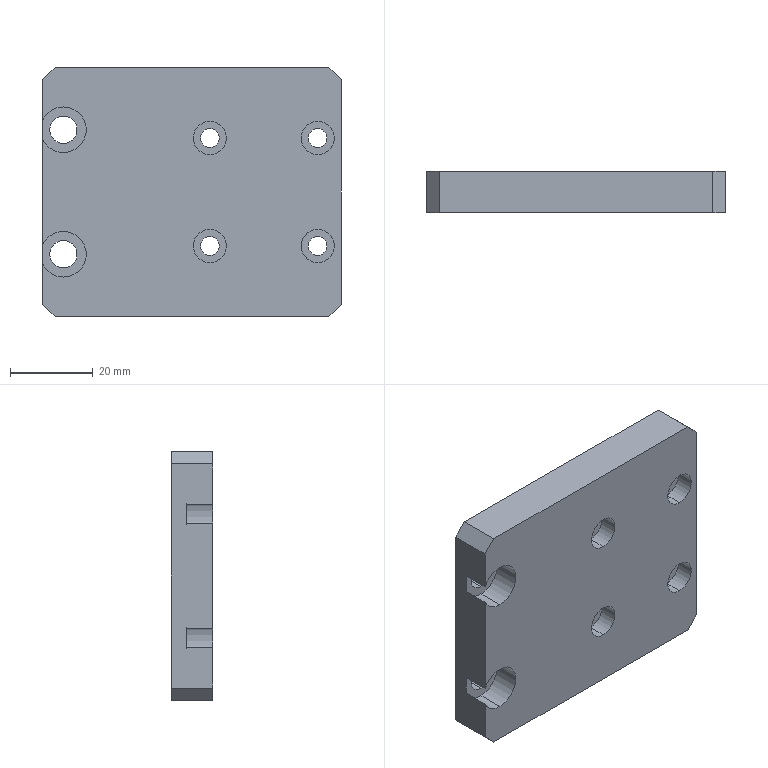Part | SolidWorks | features HoleWzd 4, Chamfer 2, Extrusion 1, ICE 1 | 1 solid | 46 faces | box 72 x 10 x 60 mm | volume 39992 mm3 | cylinder 28 | plane 16 | cone 2 | commonest cylinder face diameters 4.5 x8 8 x8 11 x6 6.6 x4 5 x2
STEP:
#1=CARTESIAN_POINT('',(5.,-44.,18.3));
#2=VERTEX_POINT('',#1);
#3=CARTESIAN_POINT('',(5.,-44.,11.7));
#4=VERTEX_POINT('',#3);
#5=CARTESIAN_POINT('',(5.,-44.,15.));
#6=DIRECTION('',(0.,-1.,0.));
#7=DIRECTION('',(0.,0.,-1.));
#8=AXIS2_PLACEMENT_3D('',#5,#6,#7);
#9=CIRCLE('',#8,3.3);
#10=EDGE_CURVE('',#2,#4,#9,.T.);
#11=ORIENTED_EDGE('',*,*,#10,.F.);
#12=CARTESIAN_POINT('',(5.,-47.6,18.3));
#13=VERTEX_POINT('',#12);
#14=CARTESIAN_POINT('',(5.,-54.,18.3));
#15=DIRECTION('',(0.,-1.,0.));
#16=VECTOR('',#15,1000.);
#17=LINE('',#14,#16);
#18=EDGE_CURVE('',#2,#13,#17,.T.);
#19=ORIENTED_EDGE('',*,*,#18,.T.);
#20=CARTESIAN_POINT('',(5.,-47.6,11.7));
#21=VERTEX_POINT('',#20);
#22=CARTESIAN_POINT('',(5.,-47.6,15.));
#23=DIRECTION('',(0.,-1.,0.));
#24=DIRECTION('',(0.,0.,-1.));
#25=AXIS2_PLACEMENT_3D('',#22,#23,#24);
#26=CIRCLE('',#25,3.3);
#27=EDGE_CURVE('',#13,#21,#26,.T.);
#28=ORIENTED_EDGE('',*,*,#27,.T.);
#29=CARTESIAN_POINT('',(5.,-54.,11.7));
#30=DIRECTION('',(0.,-1.,0.));
#31=VECTOR('',#30,1000.);
#32=LINE('',#29,#31);
#33=EDGE_CURVE('',#4,#21,#32,.T.);
#34=ORIENTED_EDGE('',*,*,#33,.F.);
#35=EDGE_LOOP('',(#11,#19,#28,#34));
#36=FACE_OUTER_BOUND('',#35,.T.);
#37=CARTESIAN_POINT('',(5.,-54.,15.));
#38=DIRECTION('',(0.,-1.,0.));
#39=DIRECTION('',(0.,0.,-1.));
#40=AXIS2_PLACEMENT_3D('',#37,#38,#39);
#41=CYLINDRICAL_SURFACE('',#40,3.3);
#42=ADVANCED_FACE('',(#36),#41,.F.);
#43=CARTESIAN_POINT('',(5.,-47.6,20.5));
#44=VERTEX_POINT('',#43);
#45=CARTESIAN_POINT('',(0.,-47.6,17.291));
#46=VERTEX_POINT('',#45);
#47=CARTESIAN_POINT('',(5.,-47.6,15.));
#48=DIRECTION('',(0.,-1.,0.));
#49=DIRECTION('',(0.,0.,-1.));
#50=AXIS2_PLACEMENT_3D('',#47,#48,#49);
#51=CIRCLE('',#50,5.5);
#52=EDGE_CURVE('',#44,#46,#51,.T.);
#53=ORIENTED_EDGE('',*,*,#52,.F.);
#54=CARTESIAN_POINT('',(5.,-54.,20.5));
#55=VERTEX_POINT('',#54);
#56=CARTESIAN_POINT('',(5.,-54.,20.5));
#57=DIRECTION('',(0.,-1.,0.));
#58=VECTOR('',#57,1000.);
#59=LINE('',#56,#58);
#60=EDGE_CURVE('',#44,#55,#59,.T.);
#61=ORIENTED_EDGE('',*,*,#60,.T.);
#62=CARTESIAN_POINT('',(0.,-54.,17.291));
#63=VERTEX_POINT('',#62);
#64=CARTESIAN_POINT('',(5.,-54.,15.));
#65=DIRECTION('',(0.,1.,0.));
#66=DIRECTION('',(0.,0.,1.));
#67=AXIS2_PLACEMENT_3D('',#64,#65,#66);
#68=CIRCLE('',#67,5.5);
#69=EDGE_CURVE('',#63,#55,#68,.T.);
#70=ORIENTED_EDGE('',*,*,#69,.F.);
#71=CARTESIAN_POINT('',(0.,-54.,17.291));
#72=DIRECTION('',(0.,-1.,0.));
#73=VECTOR('',#72,1000.);
#74=LINE('',#71,#73);
#75=EDGE_CURVE('',#46,#63,#74,.T.);
#76=ORIENTED_EDGE('',*,*,#75,.F.);
#77=EDGE_LOOP('',(#53,#61,#70,#76));
#78=FACE_OUTER_BOUND('',#77,.T.);
#79=CARTESIAN_POINT('',(5.,-54.,15.));
#80=DIRECTION('',(0.,-1.,0.));
#81=DIRECTION('',(0.,0.,-1.));
#82=AXIS2_PLACEMENT_3D('',#79,#80,#81);
#83=CYLINDRICAL_SURFACE('',#82,5.5);
#84=ADVANCED_FACE('',(#78),#83,.F.);
#85=ORIENTED_EDGE('',*,*,#60,.F.);
#86=CARTESIAN_POINT('',(5.,-47.6,9.5));
#87=VERTEX_POINT('',#86);
#88=CARTESIAN_POINT('',(5.,-47.6,15.));
#89=DIRECTION('',(0.,-1.,0.));
#90=DIRECTION('',(0.,0.,-1.));
#91=AXIS2_PLACEMENT_3D('',#88,#89,#90);
#92=CIRCLE('',#91,5.5);
#93=EDGE_CURVE('',#87,#44,#92,.T.);
#94=ORIENTED_EDGE('',*,*,#93,.F.);
#95=CARTESIAN_POINT('',(5.,-54.,9.5));
#96=VERTEX_POINT('',#95);
#97=CARTESIAN_POINT('',(5.,-54.,9.5));
#98=DIRECTION('',(0.,-1.,0.));
#99=VECTOR('',#98,1000.);
#100=LINE('',#97,#99);
#101=EDGE_CURVE('',#87,#96,#100,.T.);
#102=ORIENTED_EDGE('',*,*,#101,.T.);
#103=CARTESIAN_POINT('',(5.,-54.,15.));
#104=DIRECTION('',(0.,1.,0.));
#105=DIRECTION('',(0.,0.,1.));
#106=AXIS2_PLACEMENT_3D('',#103,#104,#105);
#107=CIRCLE('',#106,5.5);
#108=EDGE_CURVE('',#55,#96,#107,.T.);
#109=ORIENTED_EDGE('',*,*,#108,.F.);
#110=EDGE_LOOP('',(#85,#94,#102,#109));
#111=FACE_OUTER_BOUND('',#110,.T.);
#112=CARTESIAN_POINT('',(5.,-54.,15.));
#113=DIRECTION('',(0.,-1.,0.));
#114=DIRECTION('',(0.,0.,-1.));
#115=AXIS2_PLACEMENT_3D('',#112,#113,#114);
#116=CYLINDRICAL_SURFACE('',#115,5.5);
#117=ADVANCED_FACE('',(#111),#116,.F.);
#118=CARTESIAN_POINT('',(5.,-47.6,50.5));
#119=VERTEX_POINT('',#118);
#120=CARTESIAN_POINT('',(0.,-47.6,47.291));
#121=VERTEX_POINT('',#120);
#122=CARTESIAN_POINT('',(5.,-47.6,45.));
#123=DIRECTION('',(0.,-1.,0.));
#124=DIRECTION('',(0.,0.,-1.));
#125=AXIS2_PLACEMENT_3D('',#122,#123,#124);
#126=CIRCLE('',#125,5.5);
#127=EDGE_CURVE('',#119,#121,#126,.T.);
#128=ORIENTED_EDGE('',*,*,#127,.F.);
#129=CARTESIAN_POINT('',(5.,-54.,50.5));
#130=VERTEX_POINT('',#129);
#131=CARTESIAN_POINT('',(5.,-54.,50.5));
#132=DIRECTION('',(0.,-1.,0.));
#133=VECTOR('',#132,1000.);
#134=LINE('',#131,#133);
#135=EDGE_CURVE('',#119,#130,#134,.T.);
#136=ORIENTED_EDGE('',*,*,#135,.T.);
#137=CARTESIAN_POINT('',(0.,-54.,47.291));
#138=VERTEX_POINT('',#137);
#139=CARTESIAN_POINT('',(5.,-54.,45.));
#140=DIRECTION('',(0.,-1.,0.));
#141=DIRECTION('',(0.,0.,-1.));
#142=AXIS2_PLACEMENT_3D('',#139,#140,#141);
#143=CIRCLE('',#142,5.5);
#144=EDGE_CURVE('',#130,#138,#143,.T.);
#145=ORIENTED_EDGE('',*,*,#144,.T.);
#146=CARTESIAN_POINT('',(0.,-54.,47.291));
#147=DIRECTION('',(0.,-1.,0.));
#148=VECTOR('',#147,1000.);
#149=LINE('',#146,#148);
#150=EDGE_CURVE('',#121,#138,#149,.T.);
#151=ORIENTED_EDGE('',*,*,#150,.F.);
#152=EDGE_LOOP('',(#128,#136,#145,#151));
#153=FACE_OUTER_BOUND('',#152,.T.);
#154=CARTESIAN_POINT('',(5.,-54.,45.));
#155=DIRECTION('',(0.,-1.,0.));
#156=DIRECTION('',(0.,0.,-1.));
#157=AXIS2_PLACEMENT_3D('',#154,#155,#156);
#158=CYLINDRICAL_SURFACE('',#157,5.5);
#159=ADVANCED_FACE('',(#153),#158,.F.);
#160=ORIENTED_EDGE('',*,*,#135,.F.);
#161=CARTESIAN_POINT('',(5.,-47.6,39.5));
#162=VERTEX_POINT('',#161);
#163=CARTESIAN_POINT('',(5.,-47.6,45.));
#164=DIRECTION('',(0.,-1.,0.));
#165=DIRECTION('',(0.,0.,-1.));
#166=AXIS2_PLACEMENT_3D('',#163,#164,#165);
#167=CIRCLE('',#166,5.5);
#168=EDGE_CURVE('',#162,#119,#167,.T.);
#169=ORIENTED_EDGE('',*,*,#168,.F.);
#170=CARTESIAN_POINT('',(5.,-54.,39.5));
#171=VERTEX_POINT('',#170);
#172=CARTESIAN_POINT('',(5.,-54.,39.5));
#173=DIRECTION('',(0.,-1.,0.));
#174=VECTOR('',#173,1000.);
#175=LINE('',#172,#174);
#176=EDGE_CURVE('',#162,#171,#175,.T.);
#177=ORIENTED_EDGE('',*,*,#176,.T.);
#178=CARTESIAN_POINT('',(5.,-54.,45.));
#179=DIRECTION('',(0.,-1.,0.));
#180=DIRECTION('',(0.,0.,-1.));
#181=AXIS2_PLACEMENT_3D('',#178,#179,#180);
#182=CIRCLE('',#181,5.5);
#183=EDGE_CURVE('',#171,#130,#182,.T.);
#184=ORIENTED_EDGE('',*,*,#183,.T.);
#185=EDGE_LOOP('',(#160,#169,#177,#184));
#186=FACE_OUTER_BOUND('',#185,.T.);
#187=CARTESIAN_POINT('',(5.,-54.,45.));
#188=DIRECTION('',(0.,-1.,0.));
#189=DIRECTION('',(0.,0.,-1.));
#190=AXIS2_PLACEMENT_3D('',#187,#188,#189);
#191=CYLINDRICAL_SURFACE('',#190,5.5);
#192=ADVANCED_FACE('',(#186),#191,.F.);
#193=CARTESIAN_POINT('',(5.,-44.,48.3));
#194=VERTEX_POINT('',#193);
#195=CARTESIAN_POINT('',(5.,-44.,41.7));
#196=VERTEX_POINT('',#195);
#197=CARTESIAN_POINT('',(5.,-44.,45.));
#198=DIRECTION('',(0.,-1.,0.));
#199=DIRECTION('',(0.,0.,-1.));
#200=AXIS2_PLACEMENT_3D('',#197,#198,#199);
#201=CIRCLE('',#200,3.3);
#202=EDGE_CURVE('',#194,#196,#201,.T.);
#203=ORIENTED_EDGE('',*,*,#202,.F.);
#204=CARTESIAN_POINT('',(5.,-47.6,48.3));
#205=VERTEX_POINT('',#204);
#206=CARTESIAN_POINT('',(5.,-54.,48.3));
#207=DIRECTION('',(0.,-1.,0.));
#208=VECTOR('',#207,1000.);
#209=LINE('',#206,#208);
#210=EDGE_CURVE('',#194,#205,#209,.T.);
#211=ORIENTED_EDGE('',*,*,#210,.T.);
#212=CARTESIAN_POINT('',(5.,-47.6,41.7));
#213=VERTEX_POINT('',#212);
#214=CARTESIAN_POINT('',(5.,-47.6,45.));
#215=DIRECTION('',(0.,-1.,0.));
#216=DIRECTION('',(0.,0.,-1.));
#217=AXIS2_PLACEMENT_3D('',#214,#215,#216);
#218=CIRCLE('',#217,3.3);
#219=EDGE_CURVE('',#205,#213,#218,.T.);
#220=ORIENTED_EDGE('',*,*,#219,.T.);
#221=CARTESIAN_POINT('',(5.,-54.,41.7));
#222=DIRECTION('',(0.,-1.,0.));
#223=VECTOR('',#222,1000.);
#224=LINE('',#221,#223);
#225=EDGE_CURVE('',#196,#213,#224,.T.);
#226=ORIENTED_EDGE('',*,*,#225,.F.);
#227=EDGE_LOOP('',(#203,#211,#220,#226));
#228=FACE_OUTER_BOUND('',#227,.T.);
#229=CARTESIAN_POINT('',(5.,-54.,45.));
#230=DIRECTION('',(0.,-1.,0.));
#231=DIRECTION('',(0.,0.,-1.));
#232=AXIS2_PLACEMENT_3D('',#229,#230,#231);
#233=CYLINDRICAL_SURFACE('',#232,3.3);
#234=ADVANCED_FACE('',(#228),#233,.F.);
#235=CARTESIAN_POINT('',(40.3,-49.6,21.));
#236=VERTEX_POINT('',#235);
#237=CARTESIAN_POINT('',(40.3,-49.6,13.));
#238=VERTEX_POINT('',#237);
#239=CARTESIAN_POINT('',(40.3,-49.6,17.));
#240=DIRECTION('',(0.,-1.,0.));
#241=DIRECTION('',(0.,0.,-1.));
#242=AXIS2_PLACEMENT_3D('',#239,#240,#241);
#243=CIRCLE('',#242,4.);
#244=EDGE_CURVE('',#236,#238,#243,.T.);
#245=ORIENTED_EDGE('',*,*,#244,.F.);
#246=CARTESIAN_POINT('',(40.3,-54.,21.));
#247=VERTEX_POINT('',#246);
#248=CARTESIAN_POINT('',(40.3,-54.,21.));
#249=DIRECTION('',(0.,-1.,0.));
#250=VECTOR('',#249,1000.);
#251=LINE('',#248,#250);
#252=EDGE_CURVE('',#236,#247,#251,.T.);
#253=ORIENTED_EDGE('',*,*,#252,.T.);
#254=CARTESIAN_POINT('',(40.3,-54.,13.));
#255=VERTEX_POINT('',#254);
#256=CARTESIAN_POINT('',(40.3,-54.,17.));
#257=DIRECTION('',(0.,-1.,0.));
#258=DIRECTION('',(0.,0.,-1.));
#259=AXIS2_PLACEMENT_3D('',#256,#257,#258);
#260=CIRCLE('',#259,4.);
#261=EDGE_CURVE('',#247,#255,#260,.T.);
#262=ORIENTED_EDGE('',*,*,#261,.T.);
#263=CARTESIAN_POINT('',(40.3,-54.,13.));
#264=DIRECTION('',(0.,-1.,0.));
#265=VECTOR('',#264,1000.);
#266=LINE('',#263,#265);
#267=EDGE_CURVE('',#238,#255,#266,.T.);
#268=ORIENTED_EDGE('',*,*,#267,.F.);
#269=EDGE_LOOP('',(#245,#253,#262,#268));
#270=FACE_OUTER_BOUND('',#269,.T.);
#271=CARTESIAN_POINT('',(40.3,-54.,17.));
#272=DIRECTION('',(0.,-1.,0.));
#273=DIRECTION('',(0.,0.,-1.));
#274=AXIS2_PLACEMENT_3D('',#271,#272,#273);
#275=CYLINDRICAL_SURFACE('',#274,4.);
#276=ADVANCED_FACE('',(#270),#275,.F.);
#277=CARTESIAN_POINT('',(40.3,-44.,19.25));
#278=VERTEX_POINT('',#277);
#279=CARTESIAN_POINT('',(40.3,-44.,14.75));
#280=VERTEX_POINT('',#279);
#281=CARTESIAN_POINT('',(40.3,-44.,17.));
#282=DIRECTION('',(0.,-1.,0.));
#283=DIRECTION('',(0.,0.,-1.));
#284=AXIS2_PLACEMENT_3D('',#281,#282,#283);
#285=CIRCLE('',#284,2.25);
#286=EDGE_CURVE('',#278,#280,#285,.T.);
#287=ORIENTED_EDGE('',*,*,#286,.F.);
#288=CARTESIAN_POINT('',(40.3,-49.6,19.25));
#289=VERTEX_POINT('',#288);
#290=CARTESIAN_POINT('',(40.3,-54.,19.25));
#291=DIRECTION('',(0.,-1.,0.));
#292=VECTOR('',#291,1000.);
#293=LINE('',#290,#292);
#294=EDGE_CURVE('',#278,#289,#293,.T.);
#295=ORIENTED_EDGE('',*,*,#294,.T.);
#296=CARTESIAN_POINT('',(40.3,-49.6,14.75));
#297=VERTEX_POINT('',#296);
#298=CARTESIAN_POINT('',(40.3,-49.6,17.));
#299=DIRECTION('',(0.,-1.,0.));
#300=DIRECTION('',(0.,0.,-1.));
#301=AXIS2_PLACEMENT_3D('',#298,#299,#300);
#302=CIRCLE('',#301,2.25);
#303=EDGE_CURVE('',#289,#297,#302,.T.);
#304=ORIENTED_EDGE('',*,*,#303,.T.);
#305=CARTESIAN_POINT('',(40.3,-54.,14.75));
#306=DIRECTION('',(0.,-1.,0.));
#307=VECTOR('',#306,1000.);
#308=LINE('',#305,#307);
#309=EDGE_CURVE('',#280,#297,#308,.T.);
#310=ORIENTED_EDGE('',*,*,#309,.F.);
#311=EDGE_LOOP('',(#287,#295,#304,#310));
#312=FACE_OUTER_BOUND('',#311,.T.);
#313=CARTESIAN_POINT('',(40.3,-54.,17.));
#314=DIRECTION('',(0.,-1.,0.));
#315=DIRECTION('',(0.,0.,-1.));
#316=AXIS2_PLACEMENT_3D('',#313,#314,#315);
#317=CYLINDRICAL_SURFACE('',#316,2.25);
#318=ADVANCED_FACE('',(#312),#317,.F.);
#319=CARTESIAN_POINT('',(66.3,-49.6,21.));
#320=VERTEX_POINT('',#319);
#321=CARTESIAN_POINT('',(62.301,-49.6,17.074));
#322=VERTEX_POINT('',#321);
#323=CARTESIAN_POINT('',(66.3,-49.6,17.));
#324=DIRECTION('',(0.,-1.,0.));
#325=DIRECTION('',(0.,0.,-1.));
#326=AXIS2_PLACEMENT_3D('',#323,#324,#325);
#327=CIRCLE('',#326,4.);
#328=EDGE_CURVE('',#320,#322,#327,.T.);
#329=ORIENTED_EDGE('',*,*,#328,.F.);
#330=CARTESIAN_POINT('',(66.3,-54.,21.));
#331=VERTEX_POINT('',#330);
#332=CARTESIAN_POINT('',(66.3,-54.,21.));
#333=DIRECTION('',(0.,-1.,0.));
#334=VECTOR('',#333,1000.);
#335=LINE('',#332,#334);
#336=EDGE_CURVE('',#320,#331,#335,.T.);
#337=ORIENTED_EDGE('',*,*,#336,.T.);
#338=CARTESIAN_POINT('',(66.3,-54.,13.));
#339=VERTEX_POINT('',#338);
#340=CARTESIAN_POINT('',(66.3,-54.,17.));
#341=DIRECTION('',(0.,-1.,0.));
#342=DIRECTION('',(0.,0.,-1.));
#343=AXIS2_PLACEMENT_3D('',#340,#341,#342);
#344=CIRCLE('',#343,4.);
#345=EDGE_CURVE('',#331,#339,#344,.T.);
#346=ORIENTED_EDGE('',*,*,#345,.T.);
#347=CARTESIAN_POINT('',(66.3,-49.6,13.));
#348=VERTEX_POINT('',#347);
#349=CARTESIAN_POINT('',(66.3,-54.,13.));
#350=DIRECTION('',(0.,-1.,0.));
#351=VECTOR('',#350,1000.);
#352=LINE('',#349,#351);
#353=EDGE_CURVE('',#348,#339,#352,.T.);
#354=ORIENTED_EDGE('',*,*,#353,.F.);
#355=CARTESIAN_POINT('',(62.427,-49.6,16.));
#356=VERTEX_POINT('',#355);
#357=CARTESIAN_POINT('',(66.3,-49.6,17.));
#358=DIRECTION('',(0.,-1.,0.));
#359=DIRECTION('',(0.,0.,-1.));
#360=AXIS2_PLACEMENT_3D('',#357,#358,#359);
#361=CIRCLE('',#360,4.);
#362=EDGE_CURVE('',#356,#348,#361,.T.);
#363=ORIENTED_EDGE('',*,*,#362,.F.);
#364=CARTESIAN_POINT('',(62.3,-49.98,17.));
#365=VERTEX_POINT('',#364);
#366=CARTESIAN_POINT('',(62.3,-49.98,17.));
#367=CARTESIAN_POINT('',(62.3,-49.98,16.907));
#368=CARTESIAN_POINT('',(62.303,-49.972,16.815));
#369=CARTESIAN_POINT('',(62.316,-49.942,16.635));
#370=CARTESIAN_POINT('',(62.325,-49.919,16.544));
#371=CARTESIAN_POINT('',(62.349,-49.858,16.373));
#372=CARTESIAN_POINT('',(62.363,-49.819,16.291));
#373=CARTESIAN_POINT('',(62.394,-49.723,16.136));
#374=CARTESIAN_POINT('',(62.411,-49.666,16.064));
#375=CARTESIAN_POINT('',(62.427,-49.6,16.));
#376=B_SPLINE_CURVE_WITH_KNOTS('',3,(#366,#367,#368,#369,#370,#371,#372,#373,#374,#375),.UNSPECIFIED.,.F.,.F.,(4,2,2,2,4),(0.,0.0002756,0.0005511,0.0008267,0.001102),.UNSPECIFIED.);
#377=EDGE_CURVE('',#365,#356,#376,.T.);
#378=ORIENTED_EDGE('',*,*,#377,.F.);
#379=CARTESIAN_POINT('',(62.301,-49.6,17.074));
#380=CARTESIAN_POINT('',(62.3,-49.728,17.054));
#381=CARTESIAN_POINT('',(62.3,-49.854,17.03));
#382=CARTESIAN_POINT('',(62.3,-49.98,17.));
#383=B_SPLINE_CURVE_WITH_KNOTS('',3,(#379,#380,#381,#382),.UNSPECIFIED.,.F.,.F.,(4,4),(0.0001908,0.0005775),.UNSPECIFIED.);
#384=EDGE_CURVE('',#322,#365,#383,.T.);
#385=ORIENTED_EDGE('',*,*,#384,.F.);
#386=EDGE_LOOP('',(#329,#337,#346,#354,#363,#378,#385));
#387=FACE_OUTER_BOUND('',#386,.T.);
#388=CARTESIAN_POINT('',(66.3,-54.,17.));
#389=DIRECTION('',(0.,-1.,0.));
#390=DIRECTION('',(0.,0.,-1.));
#391=AXIS2_PLACEMENT_3D('',#388,#389,#390);
#392=CYLINDRICAL_SURFACE('',#391,4.);
#393=ADVANCED_FACE('',(#387),#392,.F.);
#394=CARTESIAN_POINT('',(66.3,-44.,19.25));
#395=VERTEX_POINT('',#394);
#396=CARTESIAN_POINT('',(66.3,-44.,14.75));
#397=VERTEX_POINT('',#396);
#398=CARTESIAN_POINT('',(66.3,-44.,17.));
#399=DIRECTION('',(0.,-1.,0.));
#400=DIRECTION('',(0.,0.,-1.));
#401=AXIS2_PLACEMENT_3D('',#398,#399,#400);
#402=CIRCLE('',#401,2.25);
#403=EDGE_CURVE('',#395,#397,#402,.T.);
#404=ORIENTED_EDGE('',*,*,#403,.F.);
#405=CARTESIAN_POINT('',(66.3,-49.6,19.25));
#406=VERTEX_POINT('',#405);
#407=CARTESIAN_POINT('',(66.3,-54.,19.25));
#408=DIRECTION('',(0.,-1.,0.));
#409=VECTOR('',#408,1000.);
#410=LINE('',#407,#409);
#411=EDGE_CURVE('',#395,#406,#410,.T.);
#412=ORIENTED_EDGE('',*,*,#411,.T.);
#413=CARTESIAN_POINT('',(66.3,-49.6,14.75));
#414=VERTEX_POINT('',#413);
#415=CARTESIAN_POINT('',(66.3,-49.6,17.));
#416=DIRECTION('',(0.,-1.,0.));
#417=DIRECTION('',(0.,0.,-1.));
#418=AXIS2_PLACEMENT_3D('',#415,#416,#417);
#419=CIRCLE('',#418,2.25);
#420=EDGE_CURVE('',#406,#414,#419,.T.);
#421=ORIENTED_EDGE('',*,*,#420,.T.);
#422=CARTESIAN_POINT('',(66.3,-54.,14.75));
#423=DIRECTION('',(0.,-1.,0.));
#424=VECTOR('',#423,1000.);
#425=LINE('',#422,#424);
#426=EDGE_CURVE('',#397,#414,#425,.T.);
#427=ORIENTED_EDGE('',*,*,#426,.F.);
#428=EDGE_LOOP('',(#404,#412,#421,#427));
#429=FACE_OUTER_BOUND('',#428,.T.);
#430=CARTESIAN_POINT('',(66.3,-54.,17.));
#431=DIRECTION('',(0.,-1.,0.));
#432=DIRECTION('',(0.,0.,-1.));
#433=AXIS2_PLACEMENT_3D('',#430,#431,#432);
#434=CYLINDRICAL_SURFACE('',#433,2.25);
#435=ADVANCED_FACE('',(#429),#434,.F.);
#436=CARTESIAN_POINT('',(66.3,-49.6,47.));
#437=VERTEX_POINT('',#436);
#438=CARTESIAN_POINT('',(66.3,-49.6,39.));
#439=VERTEX_POINT('',#438);
#440=CARTESIAN_POINT('',(66.3,-49.6,43.));
#441=DIRECTION('',(0.,-1.,0.));
#442=DIRECTION('',(0.,0.,-1.));
#443=AXIS2_PLACEMENT_3D('',#440,#441,#442);
#444=CIRCLE('',#443,4.);
#445=EDGE_CURVE('',#437,#439,#444,.T.);
#446=ORIENTED_EDGE('',*,*,#445,.F.);
#447=CARTESIAN_POINT('',(66.3,-54.,47.));
#448=VERTEX_POINT('',#447);
#449=CARTESIAN_POINT('',(66.3,-54.,47.));
#450=DIRECTION('',(0.,-1.,0.));
#451=VECTOR('',#450,1000.);
#452=LINE('',#449,#451);
#453=EDGE_CURVE('',#437,#448,#452,.T.);
#454=ORIENTED_EDGE('',*,*,#453,.T.);
#455=CARTESIAN_POINT('',(66.3,-54.,39.));
#456=VERTEX_POINT('',#455);
#457=CARTESIAN_POINT('',(66.3,-54.,43.));
#458=DIRECTION('',(0.,-1.,0.));
#459=DIRECTION('',(0.,0.,-1.));
#460=AXIS2_PLACEMENT_3D('',#457,#458,#459);
#461=CIRCLE('',#460,4.);
#462=EDGE_CURVE('',#448,#456,#461,.T.);
#463=ORIENTED_EDGE('',*,*,#462,.T.);
#464=CARTESIAN_POINT('',(66.3,-54.,39.));
#465=DIRECTION('',(0.,-1.,0.));
#466=VECTOR('',#465,1000.);
#467=LINE('',#464,#466);
#468=EDGE_CURVE('',#439,#456,#467,.T.);
#469=ORIENTED_EDGE('',*,*,#468,.F.);
#470=EDGE_LOOP('',(#446,#454,#463,#469));
#471=FACE_OUTER_BOUND('',#470,.T.);
#472=CARTESIAN_POINT('',(66.3,-54.,43.));
#473=DIRECTION('',(0.,-1.,0.));
#474=DIRECTION('',(0.,0.,-1.));
#475=AXIS2_PLACEMENT_3D('',#472,#473,#474);
#476=CYLINDRICAL_SURFACE('',#475,4.);
#477=ADVANCED_FACE('',(#471),#476,.F.);
#478=CARTESIAN_POINT('',(66.3,-44.,45.25));
#479=VERTEX_POINT('',#478);
#480=CARTESIAN_POINT('',(66.3,-44.,40.75));
#481=VERTEX_POINT('',#480);
#482=CARTESIAN_POINT('',(66.3,-44.,43.));
#483=DIRECTION('',(0.,-1.,0.));
#484=DIRECTION('',(0.,0.,-1.));
#485=AXIS2_PLACEMENT_3D('',#482,#483,#484);
#486=CIRCLE('',#485,2.25);
#487=EDGE_CURVE('',#479,#481,#486,.T.);
#488=ORIENTED_EDGE('',*,*,#487,.F.);
#489=CARTESIAN_POINT('',(66.3,-49.6,45.25));
#490=VERTEX_POINT('',#489);
#491=CARTESIAN_POINT('',(66.3,-54.,45.25));
#492=DIRECTION('',(0.,-1.,0.));
#493=VECTOR('',#492,1000.);
#494=LINE('',#491,#493);
#495=EDGE_CURVE('',#479,#490,#494,.T.);
#496=ORIENTED_EDGE('',*,*,#495,.T.);
#497=CARTESIAN_POINT('',(66.3,-49.6,40.75));
#498=VERTEX_POINT('',#497);
#499=CARTESIAN_POINT('',(66.3,-49.6,43.));
#500=DIRECTION('',(0.,-1.,0.));
#501=DIRECTION('',(0.,0.,-1.));
#502=AXIS2_PLACEMENT_3D('',#499,#500,#501);
#503=CIRCLE('',#502,2.25);
#504=EDGE_CURVE('',#490,#498,#503,.T.);
#505=ORIENTED_EDGE('',*,*,#504,.T.);
#506=CARTESIAN_POINT('',(66.3,-54.,40.75));
#507=DIRECTION('',(0.,-1.,0.));
#508=VECTOR('',#507,1000.);
#509=LINE('',#506,#508);
#510=EDGE_CURVE('',#481,#498,#509,.T.);
#511=ORIENTED_EDGE('',*,*,#510,.F.);
#512=EDGE_LOOP('',(#488,#496,#505,#511));
#513=FACE_OUTER_BOUND('',#512,.T.);
#514=CARTESIAN_POINT('',(66.3,-54.,43.));
#515=DIRECTION('',(0.,-1.,0.));
#516=DIRECTION('',(0.,0.,-1.));
#517=AXIS2_PLACEMENT_3D('',#514,#515,#516);
#518=CYLINDRICAL_SURFACE('',#517,2.25);
#519=ADVANCED_FACE('',(#513),#518,.F.);
#520=CARTESIAN_POINT('',(40.3,-49.6,47.));
#521=VERTEX_POINT('',#520);
#522=CARTESIAN_POINT('',(40.3,-49.6,39.));
#523=VERTEX_POINT('',#522);
#524=CARTESIAN_POINT('',(40.3,-49.6,43.));
#525=DIRECTION('',(0.,-1.,0.));
#526=DIRECTION('',(0.,0.,-1.));
#527=AXIS2_PLACEMENT_3D('',#524,#525,#526);
#528=CIRCLE('',#527,4.);
#529=EDGE_CURVE('',#521,#523,#528,.T.);
#530=ORIENTED_EDGE('',*,*,#529,.F.);
#531=CARTESIAN_POINT('',(40.3,-54.,47.));
#532=VERTEX_POINT('',#531);
#533=CARTESIAN_POINT('',(40.3,-54.,47.));
#534=DIRECTION('',(0.,-1.,0.));
#535=VECTOR('',#534,1000.);
#536=LINE('',#533,#535);
#537=EDGE_CURVE('',#521,#532,#536,.T.);
#538=ORIENTED_EDGE('',*,*,#537,.T.);
#539=CARTESIAN_POINT('',(40.3,-54.,39.));
#540=VERTEX_POINT('',#539);
#541=CARTESIAN_POINT('',(40.3,-54.,43.));
#542=DIRECTION('',(0.,-1.,0.));
#543=DIRECTION('',(0.,0.,-1.));
#544=AXIS2_PLACEMENT_3D('',#541,#542,#543);
#545=CIRCLE('',#544,4.);
#546=EDGE_CURVE('',#532,#540,#545,.T.);
#547=ORIENTED_EDGE('',*,*,#546,.T.);
#548=CARTESIAN_POINT('',(40.3,-54.,39.));
#549=DIRECTION('',(0.,-1.,0.));
#550=VECTOR('',#549,1000.);
#551=LINE('',#548,#550);
#552=EDGE_CURVE('',#523,#540,#551,.T.);
#553=ORIENTED_EDGE('',*,*,#552,.F.);
#554=EDGE_LOOP('',(#530,#538,#547,#553));
#555=FACE_OUTER_BOUND('',#554,.T.);
#556=CARTESIAN_POINT('',(40.3,-54.,43.));
#557=DIRECTION('',(0.,-1.,0.));
#558=DIRECTION('',(0.,0.,-1.));
#559=AXIS2_PLACEMENT_3D('',#556,#557,#558);
#560=CYLINDRICAL_SURFACE('',#559,4.);
#561=ADVANCED_FACE('',(#555),#560,.F.);
#562=CARTESIAN_POINT('',(40.3,-44.,45.25));
#563=VERTEX_POINT('',#562);
#564=CARTESIAN_POINT('',(40.3,-44.,40.75));
#565=VERTEX_POINT('',#564);
#566=CARTESIAN_POINT('',(40.3,-44.,43.));
#567=DIRECTION('',(0.,-1.,0.));
#568=DIRECTION('',(0.,0.,-1.));
#569=AXIS2_PLACEMENT_3D('',#566,#567,#568);
#570=CIRCLE('',#569,2.25);
#571=EDGE_CURVE('',#563,#565,#570,.T.);
#572=ORIENTED_EDGE('',*,*,#571,.F.);
#573=CARTESIAN_POINT('',(40.3,-49.6,45.25));
#574=VERTEX_POINT('',#573);
#575=CARTESIAN_POINT('',(40.3,-54.,45.25));
#576=DIRECTION('',(0.,-1.,0.));
#577=VECTOR('',#576,1000.);
#578=LINE('',#575,#577);
#579=EDGE_CURVE('',#563,#574,#578,.T.);
#580=ORIENTED_EDGE('',*,*,#579,.T.);
#581=CARTESIAN_POINT('',(40.3,-49.6,40.75));
#582=VERTEX_POINT('',#581);
#583=CARTESIAN_POINT('',(40.3,-49.6,43.));
#584=DIRECTION('',(0.,-1.,0.));
#585=DIRECTION('',(0.,0.,-1.));
#586=AXIS2_PLACEMENT_3D('',#583,#584,#585);
#587=CIRCLE('',#586,2.25);
#588=EDGE_CURVE('',#574,#582,#587,.T.);
#589=ORIENTED_EDGE('',*,*,#588,.T.);
#590=CARTESIAN_POINT('',(40.3,-54.,40.75));
#591=DIRECTION('',(0.,-1.,0.));
#592=VECTOR('',#591,1000.);
#593=LINE('',#590,#592);
#594=EDGE_CURVE('',#565,#582,#593,.T.);
#595=ORIENTED_EDGE('',*,*,#594,.F.);
#596=EDGE_LOOP('',(#572,#580,#589,#595));
#597=FACE_OUTER_BOUND('',#596,.T.);
#598=CARTESIAN_POINT('',(40.3,-54.,43.));
#599=DIRECTION('',(0.,-1.,0.));
#600=DIRECTION('',(0.,0.,-1.));
#601=AXIS2_PLACEMENT_3D('',#598,#599,#600);
#602=CYLINDRICAL_SURFACE('',#601,2.25);
#603=ADVANCED_FACE('',(#597),#602,.F.);
#604=CARTESIAN_POINT('',(62.5,-49.,17.));
#605=VERTEX_POINT('',#604);
#606=CARTESIAN_POINT('',(62.427,-49.6,17.));
#607=VERTEX_POINT('',#606);
#608=CARTESIAN_POINT('',(60.,-49.,17.));
#609=DIRECTION('',(0.,0.,-1.));
#610=DIRECTION('',(-1.,0.,0.));
#611=AXIS2_PLACEMENT_3D('',#608,#609,#610);
#612=CIRCLE('',#611,2.5);
#613=EDGE_CURVE('',#605,#607,#612,.T.);
#614=ORIENTED_EDGE('',*,*,#613,.F.);
#615=CARTESIAN_POINT('',(62.5,-49.,0.));
#616=VERTEX_POINT('',#615);
#617=CARTESIAN_POINT('',(62.5,-49.,0.));
#618=DIRECTION('',(0.,0.,-1.));
#619=VECTOR('',#618,1000.);
#620=LINE('',#617,#619);
#621=EDGE_CURVE('',#605,#616,#620,.T.);
#622=ORIENTED_EDGE('',*,*,#621,.T.);
#623=CARTESIAN_POINT('',(57.5,-49.,0.));
#624=VERTEX_POINT('',#623);
#625=CARTESIAN_POINT('',(60.,-49.,0.));
#626=DIRECTION('',(0.,0.,-1.));
#627=DIRECTION('',(-1.,0.,0.));
#628=AXIS2_PLACEMENT_3D('',#625,#626,#627);
#629=CIRCLE('',#628,2.5);
#630=EDGE_CURVE('',#616,#624,#629,.T.);
#631=ORIENTED_EDGE('',*,*,#630,.T.);
#632=CARTESIAN_POINT('',(57.5,-49.,17.));
#633=VERTEX_POINT('',#632);
#634=CARTESIAN_POINT('',(57.5,-49.,0.));
#635=DIRECTION('',(0.,0.,-1.));
#636=VECTOR('',#635,1000.);
#637=LINE('',#634,#636);
#638=EDGE_CURVE('',#633,#624,#637,.T.);
#639=ORIENTED_EDGE('',*,*,#638,.F.);
#640=CARTESIAN_POINT('',(60.,-49.,17.));
#641=DIRECTION('',(0.,0.,-1.));
#642=DIRECTION('',(-1.,0.,0.));
#643=AXIS2_PLACEMENT_3D('',#640,#641,#642);
#644=CIRCLE('',#643,2.5);
#645=EDGE_CURVE('',#365,#633,#644,.T.);
#646=ORIENTED_EDGE('',*,*,#645,.F.);
#647=ORIENTED_EDGE('',*,*,#377,.T.);
#648=CARTESIAN_POINT('',(62.427,-49.6,0.));
#649=DIRECTION('',(0.,0.,1.));
#650=VECTOR('',#649,1000.);
#651=LINE('',#648,#650);
#652=EDGE_CURVE('',#356,#607,#651,.T.);
#653=ORIENTED_EDGE('',*,*,#652,.T.);
#654=EDGE_LOOP('',(#614,#622,#631,#639,#646,#647,#653));
#655=FACE_OUTER_BOUND('',#654,.T.);
#656=CARTESIAN_POINT('',(60.,-49.,0.));
#657=DIRECTION('',(0.,0.,-1.));
#658=DIRECTION('',(-1.,0.,0.));
#659=AXIS2_PLACEMENT_3D('',#656,#657,#658);
#660=CYLINDRICAL_SURFACE('',#659,2.5);
#661=ADVANCED_FACE('',(#655),#660,.F.);
#662=CARTESIAN_POINT('',(60.,-49.,18.502));
#663=VERTEX_POINT('',#662);
#664=CARTESIAN_POINT('',(57.5,-49.,17.));
#665=DIRECTION('',(-0.8572,0.,-0.515));
#666=VECTOR('',#665,1000.);
#667=LINE('',#664,#666);
#668=EDGE_CURVE('',#663,#633,#667,.T.);
#669=ORIENTED_EDGE('',*,*,#668,.F.);
#670=CARTESIAN_POINT('',(62.5,-49.,17.));
#671=DIRECTION('',(0.8572,0.,-0.515));
#672=VECTOR('',#671,1000.);
#673=LINE('',#670,#672);
#674=EDGE_CURVE('',#663,#605,#673,.T.);
#675=ORIENTED_EDGE('',*,*,#674,.T.);
#676=ORIENTED_EDGE('',*,*,#613,.T.);
#677=CARTESIAN_POINT('',(62.427,-49.6,17.));
#678=CARTESIAN_POINT('',(62.385,-49.6,17.025));
#679=CARTESIAN_POINT('',(62.343,-49.6,17.049));
#680=CARTESIAN_POINT('',(62.301,-49.6,17.074));
#681=B_SPLINE_CURVE_WITH_KNOTS('',3,(#677,#678,#679,#680),.UNSPECIFIED.,.F.,.F.,(4,4),(0.002652,0.002798),.UNSPECIFIED.);
#682=EDGE_CURVE('',#607,#322,#681,.T.);
#683=ORIENTED_EDGE('',*,*,#682,.T.);
#684=ORIENTED_EDGE('',*,*,#384,.T.);
#685=ORIENTED_EDGE('',*,*,#645,.T.);
#686=EDGE_LOOP('',(#669,#675,#676,#683,#684,#685));
#687=FACE_OUTER_BOUND('',#686,.T.);
#688=CARTESIAN_POINT('',(60.,-49.,17.));
#689=DIRECTION('',(0.,0.,-1.));
#690=DIRECTION('',(-1.,0.,0.));
#691=AXIS2_PLACEMENT_3D('',#688,#689,#690);
#692=CONICAL_SURFACE('',#691,2.5,1.03);
#693=ADVANCED_FACE('',(#687),#692,.F.);
#694=CARTESIAN_POINT('',(40.3,-54.,17.));
#695=DIRECTION('',(0.,-1.,0.));
#696=DIRECTION('',(0.,0.,-1.));
#697=AXIS2_PLACEMENT_3D('',#694,#695,#696);
#698=CIRCLE('',#697,4.);
#699=EDGE_CURVE('',#255,#247,#698,.T.);
#700=ORIENTED_EDGE('',*,*,#699,.F.);
#701=ORIENTED_EDGE('',*,*,#261,.F.);
#702=EDGE_LOOP('',(#700,#701));
#703=FACE_BOUND('',#702,.T.);
#704=CARTESIAN_POINT('',(66.3,-54.,17.));
#705=DIRECTION('',(0.,-1.,0.));
#706=DIRECTION('',(0.,0.,-1.));
#707=AXIS2_PLACEMENT_3D('',#704,#705,#706);
#708=CIRCLE('',#707,4.);
#709=EDGE_CURVE('',#339,#331,#708,.T.);
#710=ORIENTED_EDGE('',*,*,#709,.F.);
#711=ORIENTED_EDGE('',*,*,#345,.F.);
#712=EDGE_LOOP('',(#710,#711));
#713=FACE_BOUND('',#712,.T.);
#714=CARTESIAN_POINT('',(66.3,-54.,43.));
#715=DIRECTION('',(0.,-1.,0.));
#716=DIRECTION('',(0.,0.,-1.));
#717=AXIS2_PLACEMENT_3D('',#714,#715,#716);
#718=CIRCLE('',#717,4.);
#719=EDGE_CURVE('',#456,#448,#718,.T.);
#720=ORIENTED_EDGE('',*,*,#719,.F.);
#721=ORIENTED_EDGE('',*,*,#462,.F.);
#722=EDGE_LOOP('',(#720,#721));
#723=FACE_BOUND('',#722,.T.);
#724=CARTESIAN_POINT('',(0.,-54.,42.709));
#725=VERTEX_POINT('',#724);
#726=CARTESIAN_POINT('',(0.,-54.,60.));
#727=DIRECTION('',(0.,0.,-1.));
#728=VECTOR('',#727,1000.);
#729=LINE('',#726,#728);
#730=EDGE_CURVE('',#725,#63,#729,.T.);
#731=ORIENTED_EDGE('',*,*,#730,.T.);
#732=ORIENTED_EDGE('',*,*,#69,.T.);
#733=ORIENTED_EDGE('',*,*,#108,.T.);
#734=CARTESIAN_POINT('',(0.,-54.,12.709));
#735=VERTEX_POINT('',#734);
#736=CARTESIAN_POINT('',(5.,-54.,15.));
#737=DIRECTION('',(0.,1.,0.));
#738=DIRECTION('',(0.,0.,1.));
#739=AXIS2_PLACEMENT_3D('',#736,#737,#738);
#740=CIRCLE('',#739,5.5);
#741=EDGE_CURVE('',#96,#735,#740,.T.);
#742=ORIENTED_EDGE('',*,*,#741,.T.);
#743=CARTESIAN_POINT('',(0.,-54.,3.));
#744=VERTEX_POINT('',#743);
#745=CARTESIAN_POINT('',(0.,-54.,60.));
#746=DIRECTION('',(0.,0.,-1.));
#747=VECTOR('',#746,1000.);
#748=LINE('',#745,#747);
#749=EDGE_CURVE('',#735,#744,#748,.T.);
#750=ORIENTED_EDGE('',*,*,#749,.T.);
#751=CARTESIAN_POINT('',(3.,-54.,0.));
#752=VERTEX_POINT('',#751);
#753=CARTESIAN_POINT('',(0.,-54.,3.));
#754=DIRECTION('',(0.7071,0.,-0.7071));
#755=VECTOR('',#754,1000.);
#756=LINE('',#753,#755);
#757=EDGE_CURVE('',#744,#752,#756,.T.);
#758=ORIENTED_EDGE('',*,*,#757,.T.);
#759=CARTESIAN_POINT('',(69.,-54.,0.));
#760=VERTEX_POINT('',#759);
#761=CARTESIAN_POINT('',(0.,-54.,0.));
#762=DIRECTION('',(1.,0.,0.));
#763=VECTOR('',#762,1000.);
#764=LINE('',#761,#763);
#765=EDGE_CURVE('',#752,#760,#764,.T.);
#766=ORIENTED_EDGE('',*,*,#765,.T.);
#767=CARTESIAN_POINT('',(72.,-54.,3.));
#768=VERTEX_POINT('',#767);
#769=CARTESIAN_POINT('',(72.,-54.,3.));
#770=DIRECTION('',(0.7071,0.,0.7071));
#771=VECTOR('',#770,1000.);
#772=LINE('',#769,#771);
#773=EDGE_CURVE('',#760,#768,#772,.T.);
#774=ORIENTED_EDGE('',*,*,#773,.T.);
#775=CARTESIAN_POINT('',(72.,-54.,57.));
#776=VERTEX_POINT('',#775);
#777=CARTESIAN_POINT('',(72.,-54.,60.));
#778=DIRECTION('',(0.,0.,-1.));
#779=VECTOR('',#778,1000.);
#780=LINE('',#777,#779);
#781=EDGE_CURVE('',#776,#768,#780,.T.);
#782=ORIENTED_EDGE('',*,*,#781,.F.);
#783=CARTESIAN_POINT('',(69.,-54.,60.));
#784=VERTEX_POINT('',#783);
#785=CARTESIAN_POINT('',(69.,-54.,60.));
#786=DIRECTION('',(-0.7071,0.,0.7071));
#787=VECTOR('',#786,1000.);
#788=LINE('',#785,#787);
#789=EDGE_CURVE('',#776,#784,#788,.T.);
#790=ORIENTED_EDGE('',*,*,#789,.T.);
#791=CARTESIAN_POINT('',(3.,-54.,60.));
#792=VERTEX_POINT('',#791);
#793=CARTESIAN_POINT('',(0.,-54.,60.));
#794=DIRECTION('',(1.,0.,0.));
#795=VECTOR('',#794,1000.);
#796=LINE('',#793,#795);
#797=EDGE_CURVE('',#792,#784,#796,.T.);
#798=ORIENTED_EDGE('',*,*,#797,.F.);
#799=CARTESIAN_POINT('',(0.,-54.,57.));
#800=VERTEX_POINT('',#799);
#801=CARTESIAN_POINT('',(3.,-54.,60.));
#802=DIRECTION('',(-0.7071,0.,-0.7071));
#803=VECTOR('',#802,1000.);
#804=LINE('',#801,#803);
#805=EDGE_CURVE('',#792,#800,#804,.T.);
#806=ORIENTED_EDGE('',*,*,#805,.T.);
#807=CARTESIAN_POINT('',(0.,-54.,60.));
#808=DIRECTION('',(0.,0.,-1.));
#809=VECTOR('',#808,1000.);
#810=LINE('',#807,#809);
#811=EDGE_CURVE('',#800,#138,#810,.T.);
#812=ORIENTED_EDGE('',*,*,#811,.T.);
#813=ORIENTED_EDGE('',*,*,#144,.F.);
#814=ORIENTED_EDGE('',*,*,#183,.F.);
#815=CARTESIAN_POINT('',(5.,-54.,45.));
#816=DIRECTION('',(0.,-1.,0.));
#817=DIRECTION('',(0.,0.,-1.));
#818=AXIS2_PLACEMENT_3D('',#815,#816,#817);
#819=CIRCLE('',#818,5.5);
#820=EDGE_CURVE('',#725,#171,#819,.T.);
#821=ORIENTED_EDGE('',*,*,#820,.F.);
#822=EDGE_LOOP('',(#731,#732,#733,#742,#750,#758,#766,#774,#782,#790,#798,#806,#812,#813,#814,#821));
#823=FACE_OUTER_BOUND('',#822,.T.);
#824=CARTESIAN_POINT('',(40.3,-54.,43.));
#825=DIRECTION('',(0.,-1.,0.));
#826=DIRECTION('',(0.,0.,-1.));
#827=AXIS2_PLACEMENT_3D('',#824,#825,#826);
#828=CIRCLE('',#827,4.);
#829=EDGE_CURVE('',#540,#532,#828,.T.);
#830=ORIENTED_EDGE('',*,*,#829,.F.);
#831=ORIENTED_EDGE('',*,*,#546,.F.);
#832=EDGE_LOOP('',(#830,#831));
#833=FACE_BOUND('',#832,.T.);
#834=CARTESIAN_POINT('',(0.,-54.,60.));
#835=DIRECTION('',(0.,1.,0.));
#836=DIRECTION('',(0.,0.,1.));
#837=AXIS2_PLACEMENT_3D('',#834,#835,#836);
#838=PLANE('',#837);
#839=ADVANCED_FACE('',(#703,#713,#723,#823,#833),#838,.F.);
#840=CARTESIAN_POINT('',(0.,-47.6,12.709));
#841=VERTEX_POINT('',#840);
#842=CARTESIAN_POINT('',(0.,-47.6,60.));
#843=DIRECTION('',(0.,0.,1.));
#844=VECTOR('',#843,1000.);
#845=LINE('',#842,#844);
#846=EDGE_CURVE('',#841,#46,#845,.T.);
#847=ORIENTED_EDGE('',*,*,#846,.T.);
#848=ORIENTED_EDGE('',*,*,#75,.T.);
#849=ORIENTED_EDGE('',*,*,#730,.F.);
#850=CARTESIAN_POINT('',(0.,-47.6,42.709));
#851=VERTEX_POINT('',#850);
#852=CARTESIAN_POINT('',(0.,-54.,42.709));
#853=DIRECTION('',(0.,1.,0.));
#854=VECTOR('',#853,1000.);
#855=LINE('',#852,#854);
#856=EDGE_CURVE('',#725,#851,#855,.T.);
#857=ORIENTED_EDGE('',*,*,#856,.T.);
#858=CARTESIAN_POINT('',(0.,-47.6,60.));
#859=DIRECTION('',(0.,0.,1.));
#860=VECTOR('',#859,1000.);
#861=LINE('',#858,#860);
#862=EDGE_CURVE('',#851,#121,#861,.T.);
#863=ORIENTED_EDGE('',*,*,#862,.T.);
#864=ORIENTED_EDGE('',*,*,#150,.T.);
#865=ORIENTED_EDGE('',*,*,#811,.F.);
#866=CARTESIAN_POINT('',(0.,-44.,57.));
#867=VERTEX_POINT('',#866);
#868=CARTESIAN_POINT('',(0.,0.,57.));
#869=DIRECTION('',(0.,1.,0.));
#870=VECTOR('',#869,1000.);
#871=LINE('',#868,#870);
#872=EDGE_CURVE('',#800,#867,#871,.T.);
#873=ORIENTED_EDGE('',*,*,#872,.T.);
#874=CARTESIAN_POINT('',(0.,-44.,3.));
#875=VERTEX_POINT('',#874);
#876=CARTESIAN_POINT('',(0.,-44.,0.));
#877=DIRECTION('',(0.,0.,1.));
#878=VECTOR('',#877,1000.);
#879=LINE('',#876,#878);
#880=EDGE_CURVE('',#875,#867,#879,.T.);
#881=ORIENTED_EDGE('',*,*,#880,.F.);
#882=CARTESIAN_POINT('',(0.,-54.,3.));
#883=DIRECTION('',(0.,-1.,0.));
#884=VECTOR('',#883,1000.);
#885=LINE('',#882,#884);
#886=EDGE_CURVE('',#875,#744,#885,.T.);
#887=ORIENTED_EDGE('',*,*,#886,.T.);
#888=ORIENTED_EDGE('',*,*,#749,.F.);
#889=CARTESIAN_POINT('',(0.,-54.,12.709));
#890=DIRECTION('',(0.,1.,0.));
#891=VECTOR('',#890,1000.);
#892=LINE('',#889,#891);
#893=EDGE_CURVE('',#735,#841,#892,.T.);
#894=ORIENTED_EDGE('',*,*,#893,.T.);
#895=EDGE_LOOP('',(#847,#848,#849,#857,#863,#864,#865,#873,#881,#887,#888,#894));
#896=FACE_OUTER_BOUND('',#895,.T.);
#897=CARTESIAN_POINT('',(0.,0.,60.));
#898=DIRECTION('',(1.,0.,0.));
#899=DIRECTION('',(0.,1.,0.));
#900=AXIS2_PLACEMENT_3D('',#897,#898,#899);
#901=PLANE('',#900);
#902=ADVANCED_FACE('',(#896),#901,.F.);
#903=CARTESIAN_POINT('',(72.,-44.,57.));
#904=VERTEX_POINT('',#903);
#905=CARTESIAN_POINT('',(72.,-44.,3.));
#906=VERTEX_POINT('',#905);
#907=CARTESIAN_POINT('',(72.,-44.,60.));
#908=DIRECTION('',(0.,0.,-1.));
#909=VECTOR('',#908,1000.);
#910=LINE('',#907,#909);
#911=EDGE_CURVE('',#904,#906,#910,.T.);
#912=ORIENTED_EDGE('',*,*,#911,.F.);
#913=CARTESIAN_POINT('',(72.,-54.,57.));
#914=DIRECTION('',(0.,-1.,0.));
#915=VECTOR('',#914,1000.);
#916=LINE('',#913,#915);
#917=EDGE_CURVE('',#904,#776,#916,.T.);
#918=ORIENTED_EDGE('',*,*,#917,.T.);
#919=ORIENTED_EDGE('',*,*,#781,.T.);
#920=CARTESIAN_POINT('',(72.,-44.,3.));
#921=DIRECTION('',(0.,1.,0.));
#922=VECTOR('',#921,1000.);
#923=LINE('',#920,#922);
#924=EDGE_CURVE('',#768,#906,#923,.T.);
#925=ORIENTED_EDGE('',*,*,#924,.T.);
#926=EDGE_LOOP('',(#912,#918,#919,#925));
#927=FACE_OUTER_BOUND('',#926,.T.);
#928=CARTESIAN_POINT('',(72.,-54.,60.));
#929=DIRECTION('',(-1.,0.,0.));
#930=DIRECTION('',(0.,0.,1.));
#931=AXIS2_PLACEMENT_3D('',#928,#929,#930);
#932=PLANE('',#931);
#933=ADVANCED_FACE('',(#927),#932,.F.);
#934=CARTESIAN_POINT('',(5.,-44.,15.));
#935=DIRECTION('',(0.,-1.,0.));
#936=DIRECTION('',(0.,0.,-1.));
#937=AXIS2_PLACEMENT_3D('',#934,#935,#936);
#938=CIRCLE('',#937,3.3);
#939=EDGE_CURVE('',#4,#2,#938,.T.);
#940=ORIENTED_EDGE('',*,*,#939,.T.);
#941=ORIENTED_EDGE('',*,*,#10,.T.);
#942=EDGE_LOOP('',(#940,#941));
#943=FACE_BOUND('',#942,.T.);
#944=CARTESIAN_POINT('',(5.,-44.,45.));
#945=DIRECTION('',(0.,-1.,0.));
#946=DIRECTION('',(0.,0.,-1.));
#947=AXIS2_PLACEMENT_3D('',#944,#945,#946);
#948=CIRCLE('',#947,3.3);
#949=EDGE_CURVE('',#196,#194,#948,.T.);
#950=ORIENTED_EDGE('',*,*,#949,.T.);
#951=ORIENTED_EDGE('',*,*,#202,.T.);
#952=EDGE_LOOP('',(#950,#951));
#953=FACE_BOUND('',#952,.T.);
#954=CARTESIAN_POINT('',(40.3,-44.,17.));
#955=DIRECTION('',(0.,-1.,0.));
#956=DIRECTION('',(0.,0.,-1.));
#957=AXIS2_PLACEMENT_3D('',#954,#955,#956);
#958=CIRCLE('',#957,2.25);
#959=EDGE_CURVE('',#280,#278,#958,.T.);
#960=ORIENTED_EDGE('',*,*,#959,.T.);
#961=ORIENTED_EDGE('',*,*,#286,.T.);
#962=EDGE_LOOP('',(#960,#961));
#963=FACE_BOUND('',#962,.T.);
#964=CARTESIAN_POINT('',(66.3,-44.,17.));
#965=DIRECTION('',(0.,-1.,0.));
#966=DIRECTION('',(0.,0.,-1.));
#967=AXIS2_PLACEMENT_3D('',#964,#965,#966);
#968=CIRCLE('',#967,2.25);
#969=EDGE_CURVE('',#397,#395,#968,.T.);
#970=ORIENTED_EDGE('',*,*,#969,.T.);
#971=ORIENTED_EDGE('',*,*,#403,.T.);
#972=EDGE_LOOP('',(#970,#971));
#973=FACE_BOUND('',#972,.T.);
#974=CARTESIAN_POINT('',(66.3,-44.,43.));
#975=DIRECTION('',(0.,-1.,0.));
#976=DIRECTION('',(0.,0.,-1.));
#977=AXIS2_PLACEMENT_3D('',#974,#975,#976);
#978=CIRCLE('',#977,2.25);
#979=EDGE_CURVE('',#481,#479,#978,.T.);
#980=ORIENTED_EDGE('',*,*,#979,.T.);
#981=ORIENTED_EDGE('',*,*,#487,.T.);
#982=EDGE_LOOP('',(#980,#981));
#983=FACE_BOUND('',#982,.T.);
#984=CARTESIAN_POINT('',(40.3,-44.,43.));
#985=DIRECTION('',(0.,-1.,0.));
#986=DIRECTION('',(0.,0.,-1.));
#987=AXIS2_PLACEMENT_3D('',#984,#985,#986);
#988=CIRCLE('',#987,2.25);
#989=EDGE_CURVE('',#565,#563,#988,.T.);
#990=ORIENTED_EDGE('',*,*,#989,.T.);
#991=ORIENTED_EDGE('',*,*,#571,.T.);
#992=EDGE_LOOP('',(#990,#991));
#993=FACE_BOUND('',#992,.T.);
#994=CARTESIAN_POINT('',(69.,-44.,0.));
#995=VERTEX_POINT('',#994);
#996=CARTESIAN_POINT('',(3.,-44.,0.));
#997=VERTEX_POINT('',#996);
#998=CARTESIAN_POINT('',(10.,-44.,0.));
#999=DIRECTION('',(-1.,0.,0.));
#1000=VECTOR('',#999,1000.);
#1001=LINE('',#998,#1000);
#1002=EDGE_CURVE('',#995,#997,#1001,.T.);
#1003=ORIENTED_EDGE('',*,*,#1002,.T.);
#1004=CARTESIAN_POINT('',(0.,-44.,3.));
#1005=DIRECTION('',(-0.7071,0.,0.7071));
#1006=VECTOR('',#1005,1000.);
#1007=LINE('',#1004,#1006);
#1008=EDGE_CURVE('',#997,#875,#1007,.T.);
#1009=ORIENTED_EDGE('',*,*,#1008,.T.);
#1010=ORIENTED_EDGE('',*,*,#880,.T.);
#1011=CARTESIAN_POINT('',(3.,-44.,60.));
#1012=VERTEX_POINT('',#1011);
#1013=CARTESIAN_POINT('',(3.,-44.,60.));
#1014=DIRECTION('',(0.7071,0.,0.7071));
#1015=VECTOR('',#1014,1000.);
#1016=LINE('',#1013,#1015);
#1017=EDGE_CURVE('',#867,#1012,#1016,.T.);
#1018=ORIENTED_EDGE('',*,*,#1017,.T.);
#1019=CARTESIAN_POINT('',(69.,-44.,60.));
#1020=VERTEX_POINT('',#1019);
#1021=CARTESIAN_POINT('',(10.,-44.,60.));
#1022=DIRECTION('',(-1.,0.,0.));
#1023=VECTOR('',#1022,1000.);
#1024=LINE('',#1021,#1023);
#1025=EDGE_CURVE('',#1020,#1012,#1024,.T.);
#1026=ORIENTED_EDGE('',*,*,#1025,.F.);
#1027=CARTESIAN_POINT('',(69.,-44.,60.));
#1028=DIRECTION('',(0.7071,0.,-0.7071));
#1029=VECTOR('',#1028,1000.);
#1030=LINE('',#1027,#1029);
#1031=EDGE_CURVE('',#1020,#904,#1030,.T.);
#1032=ORIENTED_EDGE('',*,*,#1031,.T.);
#1033=ORIENTED_EDGE('',*,*,#911,.T.);
#1034=CARTESIAN_POINT('',(72.,-44.,3.));
#1035=DIRECTION('',(-0.7071,0.,-0.7071));
#1036=VECTOR('',#1035,1000.);
#1037=LINE('',#1034,#1036);
#1038=EDGE_CURVE('',#906,#995,#1037,.T.);
#1039=ORIENTED_EDGE('',*,*,#1038,.T.);
#1040=EDGE_LOOP('',(#1003,#1009,#1010,#1018,#1026,#1032,#1033,#1039));
#1041=FACE_OUTER_BOUND('',#1040,.T.);
#1042=CARTESIAN_POINT('',(10.,-44.,60.));
#1043=DIRECTION('',(0.,-1.,0.));
#1044=DIRECTION('',(0.,0.,-1.));
#1045=AXIS2_PLACEMENT_3D('',#1042,#1043,#1044);
#1046=PLANE('',#1045);
#1047=ADVANCED_FACE('',(#943,#953,#963,#973,#983,#993,#1041),#1046,.F.);
#1048=ORIENTED_EDGE('',*,*,#1025,.T.);
#1049=CARTESIAN_POINT('',(3.,0.,60.));
#1050=DIRECTION('',(0.,-1.,0.));
#1051=VECTOR('',#1050,1000.);
#1052=LINE('',#1049,#1051);
#1053=EDGE_CURVE('',#1012,#792,#1052,.T.);
#1054=ORIENTED_EDGE('',*,*,#1053,.T.);
#1055=ORIENTED_EDGE('',*,*,#797,.T.);
#1056=CARTESIAN_POINT('',(69.,0.,60.));
#1057=DIRECTION('',(0.,1.,0.));
#1058=VECTOR('',#1057,1000.);
#1059=LINE('',#1056,#1058);
#1060=EDGE_CURVE('',#784,#1020,#1059,.T.);
#1061=ORIENTED_EDGE('',*,*,#1060,.T.);
#1062=EDGE_LOOP('',(#1048,#1054,#1055,#1061));
#1063=FACE_OUTER_BOUND('',#1062,.T.);
#1064=CARTESIAN_POINT('',(0.,0.,60.));
#1065=DIRECTION('',(0.,0.,-1.));
#1066=DIRECTION('',(-1.,0.,0.));
#1067=AXIS2_PLACEMENT_3D('',#1064,#1065,#1066);
#1068=PLANE('',#1067);
#1069=ADVANCED_FACE('',(#1063),#1068,.F.);
#1070=ORIENTED_EDGE('',*,*,#765,.F.);
#1071=CARTESIAN_POINT('',(3.,-44.,0.));
#1072=DIRECTION('',(0.,1.,0.));
#1073=VECTOR('',#1072,1000.);
#1074=LINE('',#1071,#1073);
#1075=EDGE_CURVE('',#752,#997,#1074,.T.);
#1076=ORIENTED_EDGE('',*,*,#1075,.T.);
#1077=ORIENTED_EDGE('',*,*,#1002,.F.);
#1078=CARTESIAN_POINT('',(69.,-54.,0.));
#1079=DIRECTION('',(0.,-1.,0.));
#1080=VECTOR('',#1079,1000.);
#1081=LINE('',#1078,#1080);
#1082=EDGE_CURVE('',#995,#760,#1081,.T.);
#1083=ORIENTED_EDGE('',*,*,#1082,.T.);
#1084=EDGE_LOOP('',(#1070,#1076,#1077,#1083));
#1085=FACE_OUTER_BOUND('',#1084,.T.);
#1086=CARTESIAN_POINT('',(60.,-49.,0.));
#1087=DIRECTION('',(0.,0.,-1.));
#1088=DIRECTION('',(-1.,0.,0.));
#1089=AXIS2_PLACEMENT_3D('',#1086,#1087,#1088);
#1090=CIRCLE('',#1089,2.5);
#1091=EDGE_CURVE('',#624,#616,#1090,.T.);
#1092=ORIENTED_EDGE('',*,*,#1091,.F.);
#1093=ORIENTED_EDGE('',*,*,#630,.F.);
#1094=EDGE_LOOP('',(#1092,#1093));
#1095=FACE_BOUND('',#1094,.T.);
#1096=CARTESIAN_POINT('',(0.,0.,0.));
#1097=DIRECTION('',(0.,0.,-1.));
#1098=DIRECTION('',(-1.,0.,0.));
#1099=AXIS2_PLACEMENT_3D('',#1096,#1097,#1098);
#1100=PLANE('',#1099);
#1101=ADVANCED_FACE('',(#1085,#1095),#1100,.T.);
#1102=ORIENTED_EDGE('',*,*,#674,.F.);
#1103=ORIENTED_EDGE('',*,*,#668,.T.);
#1104=CARTESIAN_POINT('',(60.,-49.,17.));
#1105=DIRECTION('',(0.,0.,-1.));
#1106=DIRECTION('',(-1.,0.,0.));
#1107=AXIS2_PLACEMENT_3D('',#1104,#1105,#1106);
#1108=CIRCLE('',#1107,2.5);
#1109=EDGE_CURVE('',#633,#605,#1108,.T.);
#1110=ORIENTED_EDGE('',*,*,#1109,.T.);
#1111=EDGE_LOOP('',(#1102,#1103,#1110));
#1112=FACE_OUTER_BOUND('',#1111,.T.);
#1113=CARTESIAN_POINT('',(60.,-49.,17.));
#1114=DIRECTION('',(0.,0.,-1.));
#1115=DIRECTION('',(-1.,0.,0.));
#1116=AXIS2_PLACEMENT_3D('',#1113,#1114,#1115);
#1117=CONICAL_SURFACE('',#1116,2.5,1.03);
#1118=ADVANCED_FACE('',(#1112),#1117,.F.);
#1119=ORIENTED_EDGE('',*,*,#621,.F.);
#1120=ORIENTED_EDGE('',*,*,#1109,.F.);
#1121=ORIENTED_EDGE('',*,*,#638,.T.);
#1122=ORIENTED_EDGE('',*,*,#1091,.T.);
#1123=EDGE_LOOP('',(#1119,#1120,#1121,#1122));
#1124=FACE_OUTER_BOUND('',#1123,.T.);
#1125=CARTESIAN_POINT('',(60.,-49.,0.));
#1126=DIRECTION('',(0.,0.,-1.));
#1127=DIRECTION('',(-1.,0.,0.));
#1128=AXIS2_PLACEMENT_3D('',#1125,#1126,#1127);
#1129=CYLINDRICAL_SURFACE('',#1128,2.5);
#1130=ADVANCED_FACE('',(#1124),#1129,.F.);
#1131=ORIENTED_EDGE('',*,*,#579,.F.);
#1132=ORIENTED_EDGE('',*,*,#989,.F.);
#1133=ORIENTED_EDGE('',*,*,#594,.T.);
#1134=CARTESIAN_POINT('',(40.3,-49.6,43.));
#1135=DIRECTION('',(0.,-1.,0.));
#1136=DIRECTION('',(0.,0.,-1.));
#1137=AXIS2_PLACEMENT_3D('',#1134,#1135,#1136);
#1138=CIRCLE('',#1137,2.25);
#1139=EDGE_CURVE('',#582,#574,#1138,.T.);
#1140=ORIENTED_EDGE('',*,*,#1139,.T.);
#1141=EDGE_LOOP('',(#1131,#1132,#1133,#1140));
#1142=FACE_OUTER_BOUND('',#1141,.T.);
#1143=CARTESIAN_POINT('',(40.3,-54.,43.));
#1144=DIRECTION('',(0.,-1.,0.));
#1145=DIRECTION('',(0.,0.,-1.));
#1146=AXIS2_PLACEMENT_3D('',#1143,#1144,#1145);
#1147=CYLINDRICAL_SURFACE('',#1146,2.25);
#1148=ADVANCED_FACE('',(#1142),#1147,.F.);
#1149=ORIENTED_EDGE('',*,*,#1139,.F.);
#1150=ORIENTED_EDGE('',*,*,#588,.F.);
#1151=EDGE_LOOP('',(#1149,#1150));
#1152=FACE_BOUND('',#1151,.T.);
#1153=CARTESIAN_POINT('',(40.3,-49.6,43.));
#1154=DIRECTION('',(0.,-1.,0.));
#1155=DIRECTION('',(0.,0.,-1.));
#1156=AXIS2_PLACEMENT_3D('',#1153,#1154,#1155);
#1157=CIRCLE('',#1156,4.);
#1158=EDGE_CURVE('',#523,#521,#1157,.T.);
#1159=ORIENTED_EDGE('',*,*,#1158,.T.);
#1160=ORIENTED_EDGE('',*,*,#529,.T.);
#1161=EDGE_LOOP('',(#1159,#1160));
#1162=FACE_OUTER_BOUND('',#1161,.T.);
#1163=CARTESIAN_POINT('',(42.55,-49.6,43.));
#1164=DIRECTION('',(0.,1.,0.));
#1165=DIRECTION('',(0.,0.,1.));
#1166=AXIS2_PLACEMENT_3D('',#1163,#1164,#1165);
#1167=PLANE('',#1166);
#1168=ADVANCED_FACE('',(#1152,#1162),#1167,.F.);
#1169=ORIENTED_EDGE('',*,*,#537,.F.);
#1170=ORIENTED_EDGE('',*,*,#1158,.F.);
#1171=ORIENTED_EDGE('',*,*,#552,.T.);
#1172=ORIENTED_EDGE('',*,*,#829,.T.);
#1173=EDGE_LOOP('',(#1169,#1170,#1171,#1172));
#1174=FACE_OUTER_BOUND('',#1173,.T.);
#1175=CARTESIAN_POINT('',(40.3,-54.,43.));
#1176=DIRECTION('',(0.,-1.,0.));
#1177=DIRECTION('',(0.,0.,-1.));
#1178=AXIS2_PLACEMENT_3D('',#1175,#1176,#1177);
#1179=CYLINDRICAL_SURFACE('',#1178,4.);
#1180=ADVANCED_FACE('',(#1174),#1179,.F.);
#1181=ORIENTED_EDGE('',*,*,#495,.F.);
#1182=ORIENTED_EDGE('',*,*,#979,.F.);
#1183=ORIENTED_EDGE('',*,*,#510,.T.);
#1184=CARTESIAN_POINT('',(66.3,-49.6,43.));
#1185=DIRECTION('',(0.,-1.,0.));
#1186=DIRECTION('',(0.,0.,-1.));
#1187=AXIS2_PLACEMENT_3D('',#1184,#1185,#1186);
#1188=CIRCLE('',#1187,2.25);
#1189=EDGE_CURVE('',#498,#490,#1188,.T.);
#1190=ORIENTED_EDGE('',*,*,#1189,.T.);
#1191=EDGE_LOOP('',(#1181,#1182,#1183,#1190));
#1192=FACE_OUTER_BOUND('',#1191,.T.);
#1193=CARTESIAN_POINT('',(66.3,-54.,43.));
#1194=DIRECTION('',(0.,-1.,0.));
#1195=DIRECTION('',(0.,0.,-1.));
#1196=AXIS2_PLACEMENT_3D('',#1193,#1194,#1195);
#1197=CYLINDRICAL_SURFACE('',#1196,2.25);
#1198=ADVANCED_FACE('',(#1192),#1197,.F.);
#1199=ORIENTED_EDGE('',*,*,#1189,.F.);
#1200=ORIENTED_EDGE('',*,*,#504,.F.);
#1201=EDGE_LOOP('',(#1199,#1200));
#1202=FACE_BOUND('',#1201,.T.);
#1203=CARTESIAN_POINT('',(66.3,-49.6,43.));
#1204=DIRECTION('',(0.,-1.,0.));
#1205=DIRECTION('',(0.,0.,-1.));
#1206=AXIS2_PLACEMENT_3D('',#1203,#1204,#1205);
#1207=CIRCLE('',#1206,4.);
#1208=EDGE_CURVE('',#439,#437,#1207,.T.);
#1209=ORIENTED_EDGE('',*,*,#1208,.T.);
#1210=ORIENTED_EDGE('',*,*,#445,.T.);
#1211=EDGE_LOOP('',(#1209,#1210));
#1212=FACE_OUTER_BOUND('',#1211,.T.);
#1213=CARTESIAN_POINT('',(68.55,-49.6,43.));
#1214=DIRECTION('',(0.,1.,0.));
#1215=DIRECTION('',(0.,0.,1.));
#1216=AXIS2_PLACEMENT_3D('',#1213,#1214,#1215);
#1217=PLANE('',#1216);
#1218=ADVANCED_FACE('',(#1202,#1212),#1217,.F.);
#1219=ORIENTED_EDGE('',*,*,#453,.F.);
#1220=ORIENTED_EDGE('',*,*,#1208,.F.);
#1221=ORIENTED_EDGE('',*,*,#468,.T.);
#1222=ORIENTED_EDGE('',*,*,#719,.T.);
#1223=EDGE_LOOP('',(#1219,#1220,#1221,#1222));
#1224=FACE_OUTER_BOUND('',#1223,.T.);
#1225=CARTESIAN_POINT('',(66.3,-54.,43.));
#1226=DIRECTION('',(0.,-1.,0.));
#1227=DIRECTION('',(0.,0.,-1.));
#1228=AXIS2_PLACEMENT_3D('',#1225,#1226,#1227);
#1229=CYLINDRICAL_SURFACE('',#1228,4.);
#1230=ADVANCED_FACE('',(#1224),#1229,.F.);
#1231=ORIENTED_EDGE('',*,*,#411,.F.);
#1232=ORIENTED_EDGE('',*,*,#969,.F.);
#1233=ORIENTED_EDGE('',*,*,#426,.T.);
#1234=CARTESIAN_POINT('',(66.3,-49.6,17.));
#1235=DIRECTION('',(0.,-1.,0.));
#1236=DIRECTION('',(0.,0.,-1.));
#1237=AXIS2_PLACEMENT_3D('',#1234,#1235,#1236);
#1238=CIRCLE('',#1237,2.25);
#1239=EDGE_CURVE('',#414,#406,#1238,.T.);
#1240=ORIENTED_EDGE('',*,*,#1239,.T.);
#1241=EDGE_LOOP('',(#1231,#1232,#1233,#1240));
#1242=FACE_OUTER_BOUND('',#1241,.T.);
#1243=CARTESIAN_POINT('',(66.3,-54.,17.));
#1244=DIRECTION('',(0.,-1.,0.));
#1245=DIRECTION('',(0.,0.,-1.));
#1246=AXIS2_PLACEMENT_3D('',#1243,#1244,#1245);
#1247=CYLINDRICAL_SURFACE('',#1246,2.25);
#1248=ADVANCED_FACE('',(#1242),#1247,.F.);
#1249=ORIENTED_EDGE('',*,*,#1239,.F.);
#1250=ORIENTED_EDGE('',*,*,#420,.F.);
#1251=EDGE_LOOP('',(#1249,#1250));
#1252=FACE_BOUND('',#1251,.T.);
#1253=ORIENTED_EDGE('',*,*,#362,.T.);
#1254=CARTESIAN_POINT('',(66.3,-49.6,17.));
#1255=DIRECTION('',(0.,-1.,0.));
#1256=DIRECTION('',(0.,0.,-1.));
#1257=AXIS2_PLACEMENT_3D('',#1254,#1255,#1256);
#1258=CIRCLE('',#1257,4.);
#1259=EDGE_CURVE('',#348,#320,#1258,.T.);
#1260=ORIENTED_EDGE('',*,*,#1259,.T.);
#1261=ORIENTED_EDGE('',*,*,#328,.T.);
#1262=ORIENTED_EDGE('',*,*,#682,.F.);
#1263=ORIENTED_EDGE('',*,*,#652,.F.);
#1264=EDGE_LOOP('',(#1253,#1260,#1261,#1262,#1263));
#1265=FACE_OUTER_BOUND('',#1264,.T.);
#1266=CARTESIAN_POINT('',(68.55,-49.6,17.));
#1267=DIRECTION('',(0.,1.,0.));
#1268=DIRECTION('',(0.,0.,1.));
#1269=AXIS2_PLACEMENT_3D('',#1266,#1267,#1268);
#1270=PLANE('',#1269);
#1271=ADVANCED_FACE('',(#1252,#1265),#1270,.F.);
#1272=ORIENTED_EDGE('',*,*,#336,.F.);
#1273=ORIENTED_EDGE('',*,*,#1259,.F.);
#1274=ORIENTED_EDGE('',*,*,#353,.T.);
#1275=ORIENTED_EDGE('',*,*,#709,.T.);
#1276=EDGE_LOOP('',(#1272,#1273,#1274,#1275));
#1277=FACE_OUTER_BOUND('',#1276,.T.);
#1278=CARTESIAN_POINT('',(66.3,-54.,17.));
#1279=DIRECTION('',(0.,-1.,0.));
#1280=DIRECTION('',(0.,0.,-1.));
#1281=AXIS2_PLACEMENT_3D('',#1278,#1279,#1280);
#1282=CYLINDRICAL_SURFACE('',#1281,4.);
#1283=ADVANCED_FACE('',(#1277),#1282,.F.);
#1284=ORIENTED_EDGE('',*,*,#294,.F.);
#1285=ORIENTED_EDGE('',*,*,#959,.F.);
#1286=ORIENTED_EDGE('',*,*,#309,.T.);
#1287=CARTESIAN_POINT('',(40.3,-49.6,17.));
#1288=DIRECTION('',(0.,-1.,0.));
#1289=DIRECTION('',(0.,0.,-1.));
#1290=AXIS2_PLACEMENT_3D('',#1287,#1288,#1289);
#1291=CIRCLE('',#1290,2.25);
#1292=EDGE_CURVE('',#297,#289,#1291,.T.);
#1293=ORIENTED_EDGE('',*,*,#1292,.T.);
#1294=EDGE_LOOP('',(#1284,#1285,#1286,#1293));
#1295=FACE_OUTER_BOUND('',#1294,.T.);
#1296=CARTESIAN_POINT('',(40.3,-54.,17.));
#1297=DIRECTION('',(0.,-1.,0.));
#1298=DIRECTION('',(0.,0.,-1.));
#1299=AXIS2_PLACEMENT_3D('',#1296,#1297,#1298);
#1300=CYLINDRICAL_SURFACE('',#1299,2.25);
#1301=ADVANCED_FACE('',(#1295),#1300,.F.);
#1302=ORIENTED_EDGE('',*,*,#1292,.F.);
#1303=ORIENTED_EDGE('',*,*,#303,.F.);
#1304=EDGE_LOOP('',(#1302,#1303));
#1305=FACE_BOUND('',#1304,.T.);
#1306=CARTESIAN_POINT('',(40.3,-49.6,17.));
#1307=DIRECTION('',(0.,-1.,0.));
#1308=DIRECTION('',(0.,0.,-1.));
#1309=AXIS2_PLACEMENT_3D('',#1306,#1307,#1308);
#1310=CIRCLE('',#1309,4.);
#1311=EDGE_CURVE('',#238,#236,#1310,.T.);
#1312=ORIENTED_EDGE('',*,*,#1311,.T.);
#1313=ORIENTED_EDGE('',*,*,#244,.T.);
#1314=EDGE_LOOP('',(#1312,#1313));
#1315=FACE_OUTER_BOUND('',#1314,.T.);
#1316=CARTESIAN_POINT('',(42.55,-49.6,17.));
#1317=DIRECTION('',(0.,1.,0.));
#1318=DIRECTION('',(0.,0.,1.));
#1319=AXIS2_PLACEMENT_3D('',#1316,#1317,#1318);
#1320=PLANE('',#1319);
#1321=ADVANCED_FACE('',(#1305,#1315),#1320,.F.);
#1322=ORIENTED_EDGE('',*,*,#252,.F.);
#1323=ORIENTED_EDGE('',*,*,#1311,.F.);
#1324=ORIENTED_EDGE('',*,*,#267,.T.);
#1325=ORIENTED_EDGE('',*,*,#699,.T.);
#1326=EDGE_LOOP('',(#1322,#1323,#1324,#1325));
#1327=FACE_OUTER_BOUND('',#1326,.T.);
#1328=CARTESIAN_POINT('',(40.3,-54.,17.));
#1329=DIRECTION('',(0.,-1.,0.));
#1330=DIRECTION('',(0.,0.,-1.));
#1331=AXIS2_PLACEMENT_3D('',#1328,#1329,#1330);
#1332=CYLINDRICAL_SURFACE('',#1331,4.);
#1333=ADVANCED_FACE('',(#1327),#1332,.F.);
#1334=ORIENTED_EDGE('',*,*,#789,.F.);
#1335=ORIENTED_EDGE('',*,*,#917,.F.);
#1336=ORIENTED_EDGE('',*,*,#1031,.F.);
#1337=ORIENTED_EDGE('',*,*,#1060,.F.);
#1338=EDGE_LOOP('',(#1334,#1335,#1336,#1337));
#1339=FACE_OUTER_BOUND('',#1338,.T.);
#1340=CARTESIAN_POINT('',(69.,0.,60.));
#1341=DIRECTION('',(-0.7071,0.,-0.7071));
#1342=DIRECTION('',(0.,1.,0.));
#1343=AXIS2_PLACEMENT_3D('',#1340,#1341,#1342);
#1344=PLANE('',#1343);
#1345=ADVANCED_FACE('',(#1339),#1344,.F.);
#1346=ORIENTED_EDGE('',*,*,#773,.F.);
#1347=ORIENTED_EDGE('',*,*,#1082,.F.);
#1348=ORIENTED_EDGE('',*,*,#1038,.F.);
#1349=ORIENTED_EDGE('',*,*,#924,.F.);
#1350=EDGE_LOOP('',(#1346,#1347,#1348,#1349));
#1351=FACE_OUTER_BOUND('',#1350,.T.);
#1352=CARTESIAN_POINT('',(72.,-54.,3.));
#1353=DIRECTION('',(0.7071,0.,-0.7071));
#1354=DIRECTION('',(0.,-1.,0.));
#1355=AXIS2_PLACEMENT_3D('',#1352,#1353,#1354);
#1356=PLANE('',#1355);
#1357=ADVANCED_FACE('',(#1351),#1356,.T.);
#1358=ORIENTED_EDGE('',*,*,#1008,.F.);
#1359=ORIENTED_EDGE('',*,*,#1075,.F.);
#1360=ORIENTED_EDGE('',*,*,#757,.F.);
#1361=ORIENTED_EDGE('',*,*,#886,.F.);
#1362=EDGE_LOOP('',(#1358,#1359,#1360,#1361));
#1363=FACE_OUTER_BOUND('',#1362,.T.);
#1364=CARTESIAN_POINT('',(0.,0.,3.));
#1365=DIRECTION('',(-0.7071,0.,-0.7071));
#1366=DIRECTION('',(0.,1.,0.));
#1367=AXIS2_PLACEMENT_3D('',#1364,#1365,#1366);
#1368=PLANE('',#1367);
#1369=ADVANCED_FACE('',(#1363),#1368,.T.);
#1370=ORIENTED_EDGE('',*,*,#1017,.F.);
#1371=ORIENTED_EDGE('',*,*,#872,.F.);
#1372=ORIENTED_EDGE('',*,*,#805,.F.);
#1373=ORIENTED_EDGE('',*,*,#1053,.F.);
#1374=EDGE_LOOP('',(#1370,#1371,#1372,#1373));
#1375=FACE_OUTER_BOUND('',#1374,.T.);
#1376=CARTESIAN_POINT('',(3.,0.,60.));
#1377=DIRECTION('',(0.7071,0.,-0.7071));
#1378=DIRECTION('',(0.,-1.,0.));
#1379=AXIS2_PLACEMENT_3D('',#1376,#1377,#1378);
#1380=PLANE('',#1379);
#1381=ADVANCED_FACE('',(#1375),#1380,.F.);
#1382=CARTESIAN_POINT('',(5.,-47.6,45.));
#1383=DIRECTION('',(0.,-1.,0.));
#1384=DIRECTION('',(0.,0.,-1.));
#1385=AXIS2_PLACEMENT_3D('',#1382,#1383,#1384);
#1386=CIRCLE('',#1385,3.3);
#1387=EDGE_CURVE('',#213,#205,#1386,.T.);
#1388=ORIENTED_EDGE('',*,*,#1387,.F.);
#1389=ORIENTED_EDGE('',*,*,#219,.F.);
#1390=EDGE_LOOP('',(#1388,#1389));
#1391=FACE_BOUND('',#1390,.T.);
#1392=CARTESIAN_POINT('',(5.,-47.6,45.));
#1393=DIRECTION('',(0.,-1.,0.));
#1394=DIRECTION('',(0.,0.,-1.));
#1395=AXIS2_PLACEMENT_3D('',#1392,#1393,#1394);
#1396=CIRCLE('',#1395,5.5);
#1397=EDGE_CURVE('',#851,#162,#1396,.T.);
#1398=ORIENTED_EDGE('',*,*,#1397,.T.);
#1399=ORIENTED_EDGE('',*,*,#168,.T.);
#1400=ORIENTED_EDGE('',*,*,#127,.T.);
#1401=ORIENTED_EDGE('',*,*,#862,.F.);
#1402=EDGE_LOOP('',(#1398,#1399,#1400,#1401));
#1403=FACE_OUTER_BOUND('',#1402,.T.);
#1404=CARTESIAN_POINT('',(8.3,-47.6,45.));
#1405=DIRECTION('',(0.,1.,0.));
#1406=DIRECTION('',(0.,0.,1.));
#1407=AXIS2_PLACEMENT_3D('',#1404,#1405,#1406);
#1408=PLANE('',#1407);
#1409=ADVANCED_FACE('',(#1391,#1403),#1408,.F.);
#1410=ORIENTED_EDGE('',*,*,#210,.F.);
#1411=ORIENTED_EDGE('',*,*,#949,.F.);
#1412=ORIENTED_EDGE('',*,*,#225,.T.);
#1413=ORIENTED_EDGE('',*,*,#1387,.T.);
#1414=EDGE_LOOP('',(#1410,#1411,#1412,#1413));
#1415=FACE_OUTER_BOUND('',#1414,.T.);
#1416=CARTESIAN_POINT('',(5.,-54.,45.));
#1417=DIRECTION('',(0.,-1.,0.));
#1418=DIRECTION('',(0.,0.,-1.));
#1419=AXIS2_PLACEMENT_3D('',#1416,#1417,#1418);
#1420=CYLINDRICAL_SURFACE('',#1419,3.3);
#1421=ADVANCED_FACE('',(#1415),#1420,.F.);
#1422=ORIENTED_EDGE('',*,*,#176,.F.);
#1423=ORIENTED_EDGE('',*,*,#1397,.F.);
#1424=ORIENTED_EDGE('',*,*,#856,.F.);
#1425=ORIENTED_EDGE('',*,*,#820,.T.);
#1426=EDGE_LOOP('',(#1422,#1423,#1424,#1425));
#1427=FACE_OUTER_BOUND('',#1426,.T.);
#1428=CARTESIAN_POINT('',(5.,-54.,45.));
#1429=DIRECTION('',(0.,-1.,0.));
#1430=DIRECTION('',(0.,0.,-1.));
#1431=AXIS2_PLACEMENT_3D('',#1428,#1429,#1430);
#1432=CYLINDRICAL_SURFACE('',#1431,5.5);
#1433=ADVANCED_FACE('',(#1427),#1432,.F.);
#1434=ORIENTED_EDGE('',*,*,#101,.F.);
#1435=CARTESIAN_POINT('',(5.,-47.6,15.));
#1436=DIRECTION('',(0.,-1.,0.));
#1437=DIRECTION('',(0.,0.,-1.));
#1438=AXIS2_PLACEMENT_3D('',#1435,#1436,#1437);
#1439=CIRCLE('',#1438,5.5);
#1440=EDGE_CURVE('',#841,#87,#1439,.T.);
#1441=ORIENTED_EDGE('',*,*,#1440,.F.);
#1442=ORIENTED_EDGE('',*,*,#893,.F.);
#1443=ORIENTED_EDGE('',*,*,#741,.F.);
#1444=EDGE_LOOP('',(#1434,#1441,#1442,#1443));
#1445=FACE_OUTER_BOUND('',#1444,.T.);
#1446=CARTESIAN_POINT('',(5.,-54.,15.));
#1447=DIRECTION('',(0.,-1.,0.));
#1448=DIRECTION('',(0.,0.,-1.));
#1449=AXIS2_PLACEMENT_3D('',#1446,#1447,#1448);
#1450=CYLINDRICAL_SURFACE('',#1449,5.5);
#1451=ADVANCED_FACE('',(#1445),#1450,.F.);
#1452=ORIENTED_EDGE('',*,*,#18,.F.);
#1453=ORIENTED_EDGE('',*,*,#939,.F.);
#1454=ORIENTED_EDGE('',*,*,#33,.T.);
#1455=CARTESIAN_POINT('',(5.,-47.6,15.));
#1456=DIRECTION('',(0.,-1.,0.));
#1457=DIRECTION('',(0.,0.,-1.));
#1458=AXIS2_PLACEMENT_3D('',#1455,#1456,#1457);
#1459=CIRCLE('',#1458,3.3);
#1460=EDGE_CURVE('',#21,#13,#1459,.T.);
#1461=ORIENTED_EDGE('',*,*,#1460,.T.);
#1462=EDGE_LOOP('',(#1452,#1453,#1454,#1461));
#1463=FACE_OUTER_BOUND('',#1462,.T.);
#1464=CARTESIAN_POINT('',(5.,-54.,15.));
#1465=DIRECTION('',(0.,-1.,0.));
#1466=DIRECTION('',(0.,0.,-1.));
#1467=AXIS2_PLACEMENT_3D('',#1464,#1465,#1466);
#1468=CYLINDRICAL_SURFACE('',#1467,3.3);
#1469=ADVANCED_FACE('',(#1463),#1468,.F.);
#1470=ORIENTED_EDGE('',*,*,#1460,.F.);
#1471=ORIENTED_EDGE('',*,*,#27,.F.);
#1472=EDGE_LOOP('',(#1470,#1471));
#1473=FACE_BOUND('',#1472,.T.);
#1474=ORIENTED_EDGE('',*,*,#1440,.T.);
#1475=ORIENTED_EDGE('',*,*,#93,.T.);
#1476=ORIENTED_EDGE('',*,*,#52,.T.);
#1477=ORIENTED_EDGE('',*,*,#846,.F.);
#1478=EDGE_LOOP('',(#1474,#1475,#1476,#1477));
#1479=FACE_OUTER_BOUND('',#1478,.T.);
#1480=CARTESIAN_POINT('',(8.3,-47.6,15.));
#1481=DIRECTION('',(0.,1.,0.));
#1482=DIRECTION('',(0.,0.,1.));
#1483=AXIS2_PLACEMENT_3D('',#1480,#1481,#1482);
#1484=PLANE('',#1483);
#1485=ADVANCED_FACE('',(#1473,#1479),#1484,.F.);
#1486=CLOSED_SHELL('',(#42,#84,#117,#159,#192,#234,#276,#318,#393,#435,#477,#519,#561,#603,#661,#693,#839,#902,#933,#1047,#1069,#1101,#1118,#1130,#1148,#1168,#1180,#1198,#1218,#1230,#1248,#1271,#1283,#1301,#1321,#1333,#1345,#1357,#1369,#1381,#1409,#1421,#1433,#1451,#1469,#1485));
#1487=MANIFOLD_SOLID_BREP('',#1486);
#1488=CARTESIAN_POINT('',(0.,0.,0.));
#1489=DIRECTION('',(0.,0.,1.));
#1490=DIRECTION('',(1.,0.,0.));
#1491=AXIS2_PLACEMENT_3D('',#1488,#1489,#1490);
#1492=(LENGTH_UNIT()NAMED_UNIT(*)SI_UNIT(.MILLI.,.METRE.));
#1493=UNCERTAINTY_MEASURE_WITH_UNIT(LENGTH_MEASURE(0.00001),#1492,'','');
#1494=(NAMED_UNIT(*)PLANE_ANGLE_UNIT()SI_UNIT($,.RADIAN.));
#1495=(NAMED_UNIT(*)SI_UNIT($,.STERADIAN.)SOLID_ANGLE_UNIT());
#1496=(GEOMETRIC_REPRESENTATION_CONTEXT(3)GLOBAL_UNCERTAINTY_ASSIGNED_CONTEXT((#1493))GLOBAL_UNIT_ASSIGNED_CONTEXT((#1492,#1494,#1495))REPRESENTATION_CONTEXT('',''));
#1497=ADVANCED_BREP_SHAPE_REPRESENTATION('',(#1487,#1491),#1496);